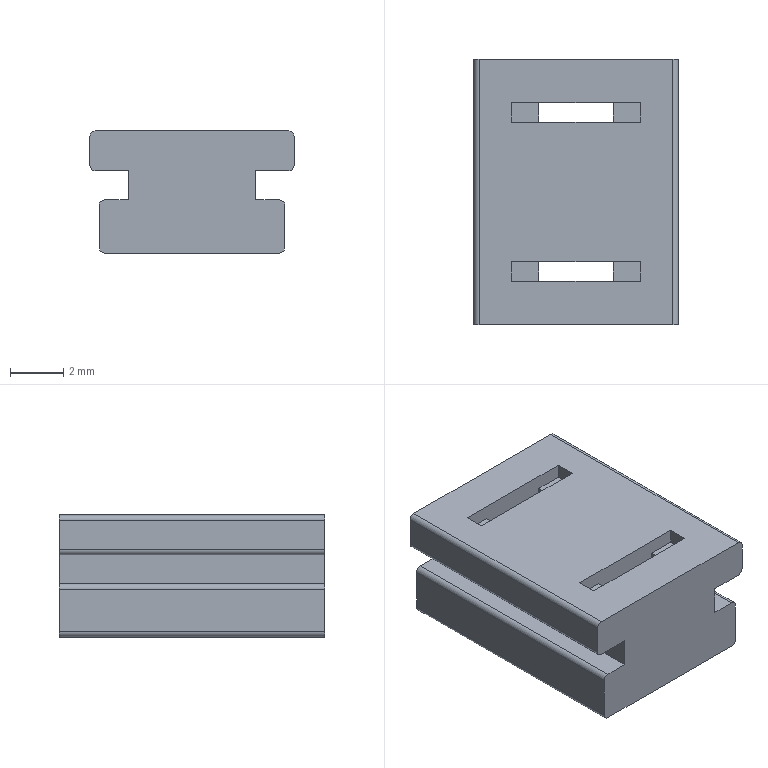Part | SolidWorks | features BaseBody 1 | 1 solid | 38 faces | box 7.7 x 10 x 4.6 mm | volume 286.602 mm3 | plane 30 | cylinder 8 | commonest cylinder face diameters 0.4 x8
STEP:
#1=CARTESIAN_POINT('',(2.425,3.375,1.5));
#2=VERTEX_POINT('',#1);
#3=CARTESIAN_POINT('',(2.425,2.625,1.5));
#4=VERTEX_POINT('',#3);
#5=CARTESIAN_POINT('',(2.425,-5.,1.5));
#6=DIRECTION('',(0.,-1.,0.));
#7=VECTOR('',#6,1000.);
#8=LINE('',#5,#7);
#9=EDGE_CURVE('',#2,#4,#8,.T.);
#10=ORIENTED_EDGE('',*,*,#9,.T.);
#11=CARTESIAN_POINT('',(-2.425,2.625,1.5));
#12=VERTEX_POINT('',#11);
#13=CARTESIAN_POINT('',(-3.85,2.625,1.5));
#14=DIRECTION('',(-1.,0.,0.));
#15=VECTOR('',#14,1000.);
#16=LINE('',#13,#15);
#17=EDGE_CURVE('',#4,#12,#16,.T.);
#18=ORIENTED_EDGE('',*,*,#17,.T.);
#19=CARTESIAN_POINT('',(-2.425,3.375,1.5));
#20=VERTEX_POINT('',#19);
#21=CARTESIAN_POINT('',(-2.425,-5.,1.5));
#22=DIRECTION('',(0.,1.,0.));
#23=VECTOR('',#22,1000.);
#24=LINE('',#21,#23);
#25=EDGE_CURVE('',#12,#20,#24,.T.);
#26=ORIENTED_EDGE('',*,*,#25,.T.);
#27=CARTESIAN_POINT('',(-3.85,3.375,1.5));
#28=DIRECTION('',(1.,0.,0.));
#29=VECTOR('',#28,1000.);
#30=LINE('',#27,#29);
#31=EDGE_CURVE('',#20,#2,#30,.T.);
#32=ORIENTED_EDGE('',*,*,#31,.T.);
#33=EDGE_LOOP('',(#10,#18,#26,#32));
#34=FACE_BOUND('',#33,.T.);
#35=CARTESIAN_POINT('',(2.425,-2.625,1.5));
#36=VERTEX_POINT('',#35);
#37=CARTESIAN_POINT('',(2.425,-3.375,1.5));
#38=VERTEX_POINT('',#37);
#39=CARTESIAN_POINT('',(2.425,-5.,1.5));
#40=DIRECTION('',(0.,-1.,0.));
#41=VECTOR('',#40,1000.);
#42=LINE('',#39,#41);
#43=EDGE_CURVE('',#36,#38,#42,.T.);
#44=ORIENTED_EDGE('',*,*,#43,.T.);
#45=CARTESIAN_POINT('',(-2.425,-3.375,1.5));
#46=VERTEX_POINT('',#45);
#47=CARTESIAN_POINT('',(-3.85,-3.375,1.5));
#48=DIRECTION('',(-1.,0.,0.));
#49=VECTOR('',#48,1000.);
#50=LINE('',#47,#49);
#51=EDGE_CURVE('',#38,#46,#50,.T.);
#52=ORIENTED_EDGE('',*,*,#51,.T.);
#53=CARTESIAN_POINT('',(-2.425,-2.625,1.5));
#54=VERTEX_POINT('',#53);
#55=CARTESIAN_POINT('',(-2.425,-5.,1.5));
#56=DIRECTION('',(0.,1.,0.));
#57=VECTOR('',#56,1000.);
#58=LINE('',#55,#57);
#59=EDGE_CURVE('',#46,#54,#58,.T.);
#60=ORIENTED_EDGE('',*,*,#59,.T.);
#61=CARTESIAN_POINT('',(-3.85,-2.625,1.5));
#62=DIRECTION('',(1.,0.,0.));
#63=VECTOR('',#62,1000.);
#64=LINE('',#61,#63);
#65=EDGE_CURVE('',#54,#36,#64,.T.);
#66=ORIENTED_EDGE('',*,*,#65,.T.);
#67=EDGE_LOOP('',(#44,#52,#60,#66));
#68=FACE_BOUND('',#67,.T.);
#69=CARTESIAN_POINT('',(-3.65,-5.,1.5));
#70=VERTEX_POINT('',#69);
#71=CARTESIAN_POINT('',(3.65,-5.,1.5));
#72=VERTEX_POINT('',#71);
#73=CARTESIAN_POINT('',(-3.85,-5.,1.5));
#74=DIRECTION('',(1.,0.,0.));
#75=VECTOR('',#74,1000.);
#76=LINE('',#73,#75);
#77=EDGE_CURVE('',#70,#72,#76,.T.);
#78=ORIENTED_EDGE('',*,*,#77,.T.);
#79=CARTESIAN_POINT('',(3.65,5.,1.5));
#80=VERTEX_POINT('',#79);
#81=CARTESIAN_POINT('',(3.65,-5.,1.5));
#82=DIRECTION('',(0.,1.,0.));
#83=VECTOR('',#82,1000.);
#84=LINE('',#81,#83);
#85=EDGE_CURVE('',#72,#80,#84,.T.);
#86=ORIENTED_EDGE('',*,*,#85,.T.);
#87=CARTESIAN_POINT('',(-3.65,5.,1.5));
#88=VERTEX_POINT('',#87);
#89=CARTESIAN_POINT('',(-3.85,5.,1.5));
#90=DIRECTION('',(-1.,0.,0.));
#91=VECTOR('',#90,1000.);
#92=LINE('',#89,#91);
#93=EDGE_CURVE('',#80,#88,#92,.T.);
#94=ORIENTED_EDGE('',*,*,#93,.T.);
#95=CARTESIAN_POINT('',(-3.65,-5.,1.5));
#96=DIRECTION('',(0.,-1.,0.));
#97=VECTOR('',#96,1000.);
#98=LINE('',#95,#97);
#99=EDGE_CURVE('',#88,#70,#98,.T.);
#100=ORIENTED_EDGE('',*,*,#99,.T.);
#101=EDGE_LOOP('',(#78,#86,#94,#100));
#102=FACE_OUTER_BOUND('',#101,.T.);
#103=CARTESIAN_POINT('',(-3.85,-5.,1.5));
#104=DIRECTION('',(0.,0.,1.));
#105=DIRECTION('',(1.,0.,0.));
#106=AXIS2_PLACEMENT_3D('',#103,#104,#105);
#107=PLANE('',#106);
#108=ADVANCED_FACE('',(#34,#68,#102),#107,.T.);
#109=CARTESIAN_POINT('',(1.4,2.625,0.95));
#110=VERTEX_POINT('',#109);
#111=CARTESIAN_POINT('',(2.425,2.625,0.95));
#112=VERTEX_POINT('',#111);
#113=CARTESIAN_POINT('',(-1.4,2.625,0.95));
#114=DIRECTION('',(1.,0.,0.));
#115=VECTOR('',#114,1000.);
#116=LINE('',#113,#115);
#117=EDGE_CURVE('',#110,#112,#116,.T.);
#118=ORIENTED_EDGE('',*,*,#117,.F.);
#119=CARTESIAN_POINT('',(1.4,2.625,-3.1));
#120=VERTEX_POINT('',#119);
#121=CARTESIAN_POINT('',(1.4,2.625,1.5));
#122=DIRECTION('',(0.,0.,1.));
#123=VECTOR('',#122,1000.);
#124=LINE('',#121,#123);
#125=EDGE_CURVE('',#120,#110,#124,.T.);
#126=ORIENTED_EDGE('',*,*,#125,.F.);
#127=CARTESIAN_POINT('',(-1.4,2.625,-3.1));
#128=VERTEX_POINT('',#127);
#129=CARTESIAN_POINT('',(-1.4,2.625,-3.1));
#130=DIRECTION('',(1.,0.,0.));
#131=VECTOR('',#130,1000.);
#132=LINE('',#129,#131);
#133=EDGE_CURVE('',#128,#120,#132,.T.);
#134=ORIENTED_EDGE('',*,*,#133,.F.);
#135=CARTESIAN_POINT('',(-1.4,2.625,0.95));
#136=VERTEX_POINT('',#135);
#137=CARTESIAN_POINT('',(-1.4,2.625,1.5));
#138=DIRECTION('',(0.,0.,-1.));
#139=VECTOR('',#138,1000.);
#140=LINE('',#137,#139);
#141=EDGE_CURVE('',#136,#128,#140,.T.);
#142=ORIENTED_EDGE('',*,*,#141,.F.);
#143=CARTESIAN_POINT('',(-2.425,2.625,0.95));
#144=VERTEX_POINT('',#143);
#145=CARTESIAN_POINT('',(-1.4,2.625,0.95));
#146=DIRECTION('',(1.,0.,0.));
#147=VECTOR('',#146,1000.);
#148=LINE('',#145,#147);
#149=EDGE_CURVE('',#144,#136,#148,.T.);
#150=ORIENTED_EDGE('',*,*,#149,.F.);
#151=CARTESIAN_POINT('',(-2.425,2.625,1.5));
#152=DIRECTION('',(0.,0.,-1.));
#153=VECTOR('',#152,1000.);
#154=LINE('',#151,#153);
#155=EDGE_CURVE('',#12,#144,#154,.T.);
#156=ORIENTED_EDGE('',*,*,#155,.F.);
#157=ORIENTED_EDGE('',*,*,#17,.F.);
#158=CARTESIAN_POINT('',(2.425,2.625,1.5));
#159=DIRECTION('',(0.,0.,1.));
#160=VECTOR('',#159,1000.);
#161=LINE('',#158,#160);
#162=EDGE_CURVE('',#112,#4,#161,.T.);
#163=ORIENTED_EDGE('',*,*,#162,.F.);
#164=EDGE_LOOP('',(#118,#126,#134,#142,#150,#156,#157,#163));
#165=FACE_OUTER_BOUND('',#164,.T.);
#166=CARTESIAN_POINT('',(-1.4,2.625,1.5));
#167=DIRECTION('',(0.,-1.,0.));
#168=DIRECTION('',(0.,0.,-1.));
#169=AXIS2_PLACEMENT_3D('',#166,#167,#168);
#170=PLANE('',#169);
#171=ADVANCED_FACE('',(#165),#170,.F.);
#172=CARTESIAN_POINT('',(2.425,3.375,0.95));
#173=VERTEX_POINT('',#172);
#174=CARTESIAN_POINT('',(2.425,2.625,0.95));
#175=DIRECTION('',(0.,1.,0.));
#176=VECTOR('',#175,1000.);
#177=LINE('',#174,#176);
#178=EDGE_CURVE('',#112,#173,#177,.T.);
#179=ORIENTED_EDGE('',*,*,#178,.F.);
#180=ORIENTED_EDGE('',*,*,#162,.T.);
#181=ORIENTED_EDGE('',*,*,#9,.F.);
#182=CARTESIAN_POINT('',(2.425,3.375,1.5));
#183=DIRECTION('',(0.,0.,1.));
#184=VECTOR('',#183,1000.);
#185=LINE('',#182,#184);
#186=EDGE_CURVE('',#173,#2,#185,.T.);
#187=ORIENTED_EDGE('',*,*,#186,.F.);
#188=EDGE_LOOP('',(#179,#180,#181,#187));
#189=FACE_OUTER_BOUND('',#188,.T.);
#190=CARTESIAN_POINT('',(2.425,2.625,1.5));
#191=DIRECTION('',(1.,0.,0.));
#192=DIRECTION('',(0.,0.,-1.));
#193=AXIS2_PLACEMENT_3D('',#190,#191,#192);
#194=PLANE('',#193);
#195=ADVANCED_FACE('',(#189),#194,.F.);
#196=CARTESIAN_POINT('',(1.4,3.375,0.95));
#197=VERTEX_POINT('',#196);
#198=CARTESIAN_POINT('',(1.4,3.375,-3.1));
#199=VERTEX_POINT('',#198);
#200=CARTESIAN_POINT('',(1.4,3.375,1.5));
#201=DIRECTION('',(0.,0.,-1.));
#202=VECTOR('',#201,1000.);
#203=LINE('',#200,#202);
#204=EDGE_CURVE('',#197,#199,#203,.T.);
#205=ORIENTED_EDGE('',*,*,#204,.F.);
#206=CARTESIAN_POINT('',(1.4,3.375,0.95));
#207=DIRECTION('',(-1.,0.,0.));
#208=VECTOR('',#207,1000.);
#209=LINE('',#206,#208);
#210=EDGE_CURVE('',#173,#197,#209,.T.);
#211=ORIENTED_EDGE('',*,*,#210,.F.);
#212=ORIENTED_EDGE('',*,*,#186,.T.);
#213=ORIENTED_EDGE('',*,*,#31,.F.);
#214=CARTESIAN_POINT('',(-2.425,3.375,0.95));
#215=VERTEX_POINT('',#214);
#216=CARTESIAN_POINT('',(-2.425,3.375,1.5));
#217=DIRECTION('',(0.,0.,1.));
#218=VECTOR('',#217,1000.);
#219=LINE('',#216,#218);
#220=EDGE_CURVE('',#215,#20,#219,.T.);
#221=ORIENTED_EDGE('',*,*,#220,.F.);
#222=CARTESIAN_POINT('',(-1.4,3.375,0.95));
#223=VERTEX_POINT('',#222);
#224=CARTESIAN_POINT('',(1.4,3.375,0.95));
#225=DIRECTION('',(-1.,0.,0.));
#226=VECTOR('',#225,1000.);
#227=LINE('',#224,#226);
#228=EDGE_CURVE('',#223,#215,#227,.T.);
#229=ORIENTED_EDGE('',*,*,#228,.F.);
#230=CARTESIAN_POINT('',(-1.4,3.375,-3.1));
#231=VERTEX_POINT('',#230);
#232=CARTESIAN_POINT('',(-1.4,3.375,1.5));
#233=DIRECTION('',(0.,0.,1.));
#234=VECTOR('',#233,1000.);
#235=LINE('',#232,#234);
#236=EDGE_CURVE('',#231,#223,#235,.T.);
#237=ORIENTED_EDGE('',*,*,#236,.F.);
#238=CARTESIAN_POINT('',(1.4,3.375,-3.1));
#239=DIRECTION('',(-1.,0.,0.));
#240=VECTOR('',#239,1000.);
#241=LINE('',#238,#240);
#242=EDGE_CURVE('',#199,#231,#241,.T.);
#243=ORIENTED_EDGE('',*,*,#242,.F.);
#244=EDGE_LOOP('',(#205,#211,#212,#213,#221,#229,#237,#243));
#245=FACE_OUTER_BOUND('',#244,.T.);
#246=CARTESIAN_POINT('',(1.4,3.375,1.5));
#247=DIRECTION('',(0.,1.,0.));
#248=DIRECTION('',(0.,0.,1.));
#249=AXIS2_PLACEMENT_3D('',#246,#247,#248);
#250=PLANE('',#249);
#251=ADVANCED_FACE('',(#245),#250,.F.);
#252=CARTESIAN_POINT('',(-2.425,3.375,0.95));
#253=DIRECTION('',(0.,-1.,0.));
#254=VECTOR('',#253,1000.);
#255=LINE('',#252,#254);
#256=EDGE_CURVE('',#215,#144,#255,.T.);
#257=ORIENTED_EDGE('',*,*,#256,.F.);
#258=ORIENTED_EDGE('',*,*,#220,.T.);
#259=ORIENTED_EDGE('',*,*,#25,.F.);
#260=ORIENTED_EDGE('',*,*,#155,.T.);
#261=EDGE_LOOP('',(#257,#258,#259,#260));
#262=FACE_OUTER_BOUND('',#261,.T.);
#263=CARTESIAN_POINT('',(-2.425,3.375,1.5));
#264=DIRECTION('',(-1.,0.,0.));
#265=DIRECTION('',(0.,0.,1.));
#266=AXIS2_PLACEMENT_3D('',#263,#264,#265);
#267=PLANE('',#266);
#268=ADVANCED_FACE('',(#262),#267,.F.);
#269=CARTESIAN_POINT('',(1.4,-3.375,0.95));
#270=VERTEX_POINT('',#269);
#271=CARTESIAN_POINT('',(2.425,-3.375,0.95));
#272=VERTEX_POINT('',#271);
#273=CARTESIAN_POINT('',(-1.4,-3.375,0.95));
#274=DIRECTION('',(1.,0.,0.));
#275=VECTOR('',#274,1000.);
#276=LINE('',#273,#275);
#277=EDGE_CURVE('',#270,#272,#276,.T.);
#278=ORIENTED_EDGE('',*,*,#277,.F.);
#279=CARTESIAN_POINT('',(1.4,-3.375,-3.1));
#280=VERTEX_POINT('',#279);
#281=CARTESIAN_POINT('',(1.4,-3.375,1.5));
#282=DIRECTION('',(0.,0.,1.));
#283=VECTOR('',#282,1000.);
#284=LINE('',#281,#283);
#285=EDGE_CURVE('',#280,#270,#284,.T.);
#286=ORIENTED_EDGE('',*,*,#285,.F.);
#287=CARTESIAN_POINT('',(-1.4,-3.375,-3.1));
#288=VERTEX_POINT('',#287);
#289=CARTESIAN_POINT('',(-1.4,-3.375,-3.1));
#290=DIRECTION('',(1.,0.,0.));
#291=VECTOR('',#290,1000.);
#292=LINE('',#289,#291);
#293=EDGE_CURVE('',#288,#280,#292,.T.);
#294=ORIENTED_EDGE('',*,*,#293,.F.);
#295=CARTESIAN_POINT('',(-1.4,-3.375,0.95));
#296=VERTEX_POINT('',#295);
#297=CARTESIAN_POINT('',(-1.4,-3.375,1.5));
#298=DIRECTION('',(0.,0.,-1.));
#299=VECTOR('',#298,1000.);
#300=LINE('',#297,#299);
#301=EDGE_CURVE('',#296,#288,#300,.T.);
#302=ORIENTED_EDGE('',*,*,#301,.F.);
#303=CARTESIAN_POINT('',(-2.425,-3.375,0.95));
#304=VERTEX_POINT('',#303);
#305=CARTESIAN_POINT('',(-1.4,-3.375,0.95));
#306=DIRECTION('',(1.,0.,0.));
#307=VECTOR('',#306,1000.);
#308=LINE('',#305,#307);
#309=EDGE_CURVE('',#304,#296,#308,.T.);
#310=ORIENTED_EDGE('',*,*,#309,.F.);
#311=CARTESIAN_POINT('',(-2.425,-3.375,1.5));
#312=DIRECTION('',(0.,0.,-1.));
#313=VECTOR('',#312,1000.);
#314=LINE('',#311,#313);
#315=EDGE_CURVE('',#46,#304,#314,.T.);
#316=ORIENTED_EDGE('',*,*,#315,.F.);
#317=ORIENTED_EDGE('',*,*,#51,.F.);
#318=CARTESIAN_POINT('',(2.425,-3.375,1.5));
#319=DIRECTION('',(0.,0.,1.));
#320=VECTOR('',#319,1000.);
#321=LINE('',#318,#320);
#322=EDGE_CURVE('',#272,#38,#321,.T.);
#323=ORIENTED_EDGE('',*,*,#322,.F.);
#324=EDGE_LOOP('',(#278,#286,#294,#302,#310,#316,#317,#323));
#325=FACE_OUTER_BOUND('',#324,.T.);
#326=CARTESIAN_POINT('',(-1.4,-3.375,1.5));
#327=DIRECTION('',(0.,-1.,0.));
#328=DIRECTION('',(0.,0.,-1.));
#329=AXIS2_PLACEMENT_3D('',#326,#327,#328);
#330=PLANE('',#329);
#331=ADVANCED_FACE('',(#325),#330,.F.);
#332=CARTESIAN_POINT('',(2.425,-2.625,0.95));
#333=VERTEX_POINT('',#332);
#334=CARTESIAN_POINT('',(2.425,-3.375,0.95));
#335=DIRECTION('',(0.,1.,0.));
#336=VECTOR('',#335,1000.);
#337=LINE('',#334,#336);
#338=EDGE_CURVE('',#272,#333,#337,.T.);
#339=ORIENTED_EDGE('',*,*,#338,.F.);
#340=ORIENTED_EDGE('',*,*,#322,.T.);
#341=ORIENTED_EDGE('',*,*,#43,.F.);
#342=CARTESIAN_POINT('',(2.425,-2.625,1.5));
#343=DIRECTION('',(0.,0.,1.));
#344=VECTOR('',#343,1000.);
#345=LINE('',#342,#344);
#346=EDGE_CURVE('',#333,#36,#345,.T.);
#347=ORIENTED_EDGE('',*,*,#346,.F.);
#348=EDGE_LOOP('',(#339,#340,#341,#347));
#349=FACE_OUTER_BOUND('',#348,.T.);
#350=CARTESIAN_POINT('',(2.425,-3.375,1.5));
#351=DIRECTION('',(1.,0.,0.));
#352=DIRECTION('',(0.,0.,-1.));
#353=AXIS2_PLACEMENT_3D('',#350,#351,#352);
#354=PLANE('',#353);
#355=ADVANCED_FACE('',(#349),#354,.F.);
#356=CARTESIAN_POINT('',(1.4,-2.625,0.95));
#357=VERTEX_POINT('',#356);
#358=CARTESIAN_POINT('',(1.4,-2.625,-3.1));
#359=VERTEX_POINT('',#358);
#360=CARTESIAN_POINT('',(1.4,-2.625,1.5));
#361=DIRECTION('',(0.,0.,-1.));
#362=VECTOR('',#361,1000.);
#363=LINE('',#360,#362);
#364=EDGE_CURVE('',#357,#359,#363,.T.);
#365=ORIENTED_EDGE('',*,*,#364,.F.);
#366=CARTESIAN_POINT('',(1.4,-2.625,0.95));
#367=DIRECTION('',(-1.,0.,0.));
#368=VECTOR('',#367,1000.);
#369=LINE('',#366,#368);
#370=EDGE_CURVE('',#333,#357,#369,.T.);
#371=ORIENTED_EDGE('',*,*,#370,.F.);
#372=ORIENTED_EDGE('',*,*,#346,.T.);
#373=ORIENTED_EDGE('',*,*,#65,.F.);
#374=CARTESIAN_POINT('',(-2.425,-2.625,0.95));
#375=VERTEX_POINT('',#374);
#376=CARTESIAN_POINT('',(-2.425,-2.625,1.5));
#377=DIRECTION('',(0.,0.,1.));
#378=VECTOR('',#377,1000.);
#379=LINE('',#376,#378);
#380=EDGE_CURVE('',#375,#54,#379,.T.);
#381=ORIENTED_EDGE('',*,*,#380,.F.);
#382=CARTESIAN_POINT('',(-1.4,-2.625,0.95));
#383=VERTEX_POINT('',#382);
#384=CARTESIAN_POINT('',(1.4,-2.625,0.95));
#385=DIRECTION('',(-1.,0.,0.));
#386=VECTOR('',#385,1000.);
#387=LINE('',#384,#386);
#388=EDGE_CURVE('',#383,#375,#387,.T.);
#389=ORIENTED_EDGE('',*,*,#388,.F.);
#390=CARTESIAN_POINT('',(-1.4,-2.625,-3.1));
#391=VERTEX_POINT('',#390);
#392=CARTESIAN_POINT('',(-1.4,-2.625,1.5));
#393=DIRECTION('',(0.,0.,1.));
#394=VECTOR('',#393,1000.);
#395=LINE('',#392,#394);
#396=EDGE_CURVE('',#391,#383,#395,.T.);
#397=ORIENTED_EDGE('',*,*,#396,.F.);
#398=CARTESIAN_POINT('',(1.4,-2.625,-3.1));
#399=DIRECTION('',(-1.,0.,0.));
#400=VECTOR('',#399,1000.);
#401=LINE('',#398,#400);
#402=EDGE_CURVE('',#359,#391,#401,.T.);
#403=ORIENTED_EDGE('',*,*,#402,.F.);
#404=EDGE_LOOP('',(#365,#371,#372,#373,#381,#389,#397,#403));
#405=FACE_OUTER_BOUND('',#404,.T.);
#406=CARTESIAN_POINT('',(1.4,-2.625,1.5));
#407=DIRECTION('',(0.,1.,0.));
#408=DIRECTION('',(0.,0.,1.));
#409=AXIS2_PLACEMENT_3D('',#406,#407,#408);
#410=PLANE('',#409);
#411=ADVANCED_FACE('',(#405),#410,.F.);
#412=CARTESIAN_POINT('',(-2.425,-2.625,0.95));
#413=DIRECTION('',(0.,-1.,0.));
#414=VECTOR('',#413,1000.);
#415=LINE('',#412,#414);
#416=EDGE_CURVE('',#375,#304,#415,.T.);
#417=ORIENTED_EDGE('',*,*,#416,.F.);
#418=ORIENTED_EDGE('',*,*,#380,.T.);
#419=ORIENTED_EDGE('',*,*,#59,.F.);
#420=ORIENTED_EDGE('',*,*,#315,.T.);
#421=EDGE_LOOP('',(#417,#418,#419,#420));
#422=FACE_OUTER_BOUND('',#421,.T.);
#423=CARTESIAN_POINT('',(-2.425,-2.625,1.5));
#424=DIRECTION('',(-1.,0.,0.));
#425=DIRECTION('',(0.,0.,1.));
#426=AXIS2_PLACEMENT_3D('',#423,#424,#425);
#427=PLANE('',#426);
#428=ADVANCED_FACE('',(#422),#427,.F.);
#429=ORIENTED_EDGE('',*,*,#85,.F.);
#430=CARTESIAN_POINT('',(3.85,-5.,1.3));
#431=VERTEX_POINT('',#430);
#432=CARTESIAN_POINT('',(3.65,-5.,1.3));
#433=DIRECTION('',(0.,1.,0.));
#434=DIRECTION('',(0.,0.,-1.));
#435=AXIS2_PLACEMENT_3D('',#432,#433,#434);
#436=CIRCLE('',#435,0.2);
#437=EDGE_CURVE('',#72,#431,#436,.T.);
#438=ORIENTED_EDGE('',*,*,#437,.T.);
#439=CARTESIAN_POINT('',(3.85,5.,1.3));
#440=VERTEX_POINT('',#439);
#441=CARTESIAN_POINT('',(3.85,18.036,1.3));
#442=DIRECTION('',(0.,1.,0.));
#443=VECTOR('',#442,1000.);
#444=LINE('',#441,#443);
#445=EDGE_CURVE('',#431,#440,#444,.T.);
#446=ORIENTED_EDGE('',*,*,#445,.T.);
#447=CARTESIAN_POINT('',(3.65,5.,1.3));
#448=DIRECTION('',(0.,-1.,0.));
#449=DIRECTION('',(0.,0.,-1.));
#450=AXIS2_PLACEMENT_3D('',#447,#448,#449);
#451=CIRCLE('',#450,0.2);
#452=EDGE_CURVE('',#440,#80,#451,.T.);
#453=ORIENTED_EDGE('',*,*,#452,.T.);
#454=EDGE_LOOP('',(#429,#438,#446,#453));
#455=FACE_OUTER_BOUND('',#454,.T.);
#456=CARTESIAN_POINT('',(3.65,18.036,1.3));
#457=DIRECTION('',(0.,-1.,0.));
#458=DIRECTION('',(0.,0.,-1.));
#459=AXIS2_PLACEMENT_3D('',#456,#457,#458);
#460=CYLINDRICAL_SURFACE('',#459,0.2);
#461=ADVANCED_FACE('',(#455),#460,.T.);
#462=CARTESIAN_POINT('',(3.5,-5.,-2.9));
#463=VERTEX_POINT('',#462);
#464=CARTESIAN_POINT('',(3.3,-5.,-3.1));
#465=VERTEX_POINT('',#464);
#466=CARTESIAN_POINT('',(3.3,-5.,-2.9));
#467=DIRECTION('',(0.,1.,0.));
#468=DIRECTION('',(0.,0.,-1.));
#469=AXIS2_PLACEMENT_3D('',#466,#467,#468);
#470=CIRCLE('',#469,0.2);
#471=EDGE_CURVE('',#463,#465,#470,.T.);
#472=ORIENTED_EDGE('',*,*,#471,.F.);
#473=CARTESIAN_POINT('',(3.5,-5.,-1.3));
#474=VERTEX_POINT('',#473);
#475=CARTESIAN_POINT('',(3.5,-5.,-1.1));
#476=DIRECTION('',(0.,0.,-1.));
#477=VECTOR('',#476,1000.);
#478=LINE('',#475,#477);
#479=EDGE_CURVE('',#474,#463,#478,.T.);
#480=ORIENTED_EDGE('',*,*,#479,.F.);
#481=CARTESIAN_POINT('',(3.3,-5.,-1.1));
#482=VERTEX_POINT('',#481);
#483=CARTESIAN_POINT('',(3.3,-5.,-1.3));
#484=DIRECTION('',(0.,1.,0.));
#485=DIRECTION('',(0.,0.,-1.));
#486=AXIS2_PLACEMENT_3D('',#483,#484,#485);
#487=CIRCLE('',#486,0.2);
#488=EDGE_CURVE('',#482,#474,#487,.T.);
#489=ORIENTED_EDGE('',*,*,#488,.F.);
#490=CARTESIAN_POINT('',(2.4,-5.,-1.1));
#491=VERTEX_POINT('',#490);
#492=CARTESIAN_POINT('',(-3.5,-5.,-1.1));
#493=DIRECTION('',(1.,0.,0.));
#494=VECTOR('',#493,1000.);
#495=LINE('',#492,#494);
#496=EDGE_CURVE('',#491,#482,#495,.T.);
#497=ORIENTED_EDGE('',*,*,#496,.F.);
#498=CARTESIAN_POINT('',(2.4,-5.,0.));
#499=VERTEX_POINT('',#498);
#500=CARTESIAN_POINT('',(2.4,-5.,0.));
#501=DIRECTION('',(0.,0.,-1.));
#502=VECTOR('',#501,1000.);
#503=LINE('',#500,#502);
#504=EDGE_CURVE('',#499,#491,#503,.T.);
#505=ORIENTED_EDGE('',*,*,#504,.F.);
#506=CARTESIAN_POINT('',(3.65,-5.,0.));
#507=VERTEX_POINT('',#506);
#508=CARTESIAN_POINT('',(3.85,-5.,0.));
#509=DIRECTION('',(-1.,0.,0.));
#510=VECTOR('',#509,1000.);
#511=LINE('',#508,#510);
#512=EDGE_CURVE('',#507,#499,#511,.T.);
#513=ORIENTED_EDGE('',*,*,#512,.F.);
#514=CARTESIAN_POINT('',(3.85,-5.,0.2));
#515=VERTEX_POINT('',#514);
#516=CARTESIAN_POINT('',(3.65,-5.,0.2));
#517=DIRECTION('',(0.,1.,0.));
#518=DIRECTION('',(0.,0.,-1.));
#519=AXIS2_PLACEMENT_3D('',#516,#517,#518);
#520=CIRCLE('',#519,0.2);
#521=EDGE_CURVE('',#515,#507,#520,.T.);
#522=ORIENTED_EDGE('',*,*,#521,.F.);
#523=CARTESIAN_POINT('',(3.85,-5.,0.));
#524=DIRECTION('',(0.,0.,-1.));
#525=VECTOR('',#524,1000.);
#526=LINE('',#523,#525);
#527=EDGE_CURVE('',#431,#515,#526,.T.);
#528=ORIENTED_EDGE('',*,*,#527,.F.);
#529=ORIENTED_EDGE('',*,*,#437,.F.);
#530=ORIENTED_EDGE('',*,*,#77,.F.);
#531=CARTESIAN_POINT('',(-3.85,-5.,1.3));
#532=VERTEX_POINT('',#531);
#533=CARTESIAN_POINT('',(-3.65,-5.,1.3));
#534=DIRECTION('',(0.,1.,0.));
#535=DIRECTION('',(0.,0.,-1.));
#536=AXIS2_PLACEMENT_3D('',#533,#534,#535);
#537=CIRCLE('',#536,0.2);
#538=EDGE_CURVE('',#532,#70,#537,.T.);
#539=ORIENTED_EDGE('',*,*,#538,.F.);
#540=CARTESIAN_POINT('',(-3.85,-5.,0.2));
#541=VERTEX_POINT('',#540);
#542=CARTESIAN_POINT('',(-3.85,-5.,0.));
#543=DIRECTION('',(0.,0.,1.));
#544=VECTOR('',#543,1000.);
#545=LINE('',#542,#544);
#546=EDGE_CURVE('',#541,#532,#545,.T.);
#547=ORIENTED_EDGE('',*,*,#546,.F.);
#548=CARTESIAN_POINT('',(-3.65,-5.,0.));
#549=VERTEX_POINT('',#548);
#550=CARTESIAN_POINT('',(-3.65,-5.,0.2));
#551=DIRECTION('',(0.,1.,0.));
#552=DIRECTION('',(0.,0.,-1.));
#553=AXIS2_PLACEMENT_3D('',#550,#551,#552);
#554=CIRCLE('',#553,0.2);
#555=EDGE_CURVE('',#549,#541,#554,.T.);
#556=ORIENTED_EDGE('',*,*,#555,.F.);
#557=CARTESIAN_POINT('',(-2.4,-5.,0.));
#558=VERTEX_POINT('',#557);
#559=CARTESIAN_POINT('',(3.85,-5.,0.));
#560=DIRECTION('',(-1.,0.,0.));
#561=VECTOR('',#560,1000.);
#562=LINE('',#559,#561);
#563=EDGE_CURVE('',#558,#549,#562,.T.);
#564=ORIENTED_EDGE('',*,*,#563,.F.);
#565=CARTESIAN_POINT('',(-2.4,-5.,-1.1));
#566=VERTEX_POINT('',#565);
#567=CARTESIAN_POINT('',(-2.4,-5.,-1.1));
#568=DIRECTION('',(0.,0.,1.));
#569=VECTOR('',#568,1000.);
#570=LINE('',#567,#569);
#571=EDGE_CURVE('',#566,#558,#570,.T.);
#572=ORIENTED_EDGE('',*,*,#571,.F.);
#573=CARTESIAN_POINT('',(-3.3,-5.,-1.1));
#574=VERTEX_POINT('',#573);
#575=CARTESIAN_POINT('',(-3.5,-5.,-1.1));
#576=DIRECTION('',(1.,0.,0.));
#577=VECTOR('',#576,1000.);
#578=LINE('',#575,#577);
#579=EDGE_CURVE('',#574,#566,#578,.T.);
#580=ORIENTED_EDGE('',*,*,#579,.F.);
#581=CARTESIAN_POINT('',(-3.5,-5.,-1.3));
#582=VERTEX_POINT('',#581);
#583=CARTESIAN_POINT('',(-3.3,-5.,-1.3));
#584=DIRECTION('',(0.,1.,0.));
#585=DIRECTION('',(0.,0.,-1.));
#586=AXIS2_PLACEMENT_3D('',#583,#584,#585);
#587=CIRCLE('',#586,0.2);
#588=EDGE_CURVE('',#582,#574,#587,.T.);
#589=ORIENTED_EDGE('',*,*,#588,.F.);
#590=CARTESIAN_POINT('',(-3.5,-5.,-2.9));
#591=VERTEX_POINT('',#590);
#592=CARTESIAN_POINT('',(-3.5,-5.,-3.1));
#593=DIRECTION('',(0.,0.,1.));
#594=VECTOR('',#593,1000.);
#595=LINE('',#592,#594);
#596=EDGE_CURVE('',#591,#582,#595,.T.);
#597=ORIENTED_EDGE('',*,*,#596,.F.);
#598=CARTESIAN_POINT('',(-3.3,-5.,-3.1));
#599=VERTEX_POINT('',#598);
#600=CARTESIAN_POINT('',(-3.3,-5.,-2.9));
#601=DIRECTION('',(0.,1.,0.));
#602=DIRECTION('',(0.,0.,-1.));
#603=AXIS2_PLACEMENT_3D('',#600,#601,#602);
#604=CIRCLE('',#603,0.2);
#605=EDGE_CURVE('',#599,#591,#604,.T.);
#606=ORIENTED_EDGE('',*,*,#605,.F.);
#607=CARTESIAN_POINT('',(0.,-5.,-3.1));
#608=DIRECTION('',(-1.,0.,0.));
#609=VECTOR('',#608,1000.);
#610=LINE('',#607,#609);
#611=EDGE_CURVE('',#465,#599,#610,.T.);
#612=ORIENTED_EDGE('',*,*,#611,.F.);
#613=EDGE_LOOP('',(#472,#480,#489,#497,#505,#513,#522,#528,#529,#530,#539,#547,#556,#564,#572,#580,#589,#597,#606,#612));
#614=FACE_OUTER_BOUND('',#613,.T.);
#615=CARTESIAN_POINT('',(0.,-5.,0.));
#616=DIRECTION('',(0.,1.,0.));
#617=DIRECTION('',(0.,0.,1.));
#618=AXIS2_PLACEMENT_3D('',#615,#616,#617);
#619=PLANE('',#618);
#620=ADVANCED_FACE('',(#614),#619,.F.);
#621=CARTESIAN_POINT('',(-3.85,5.,1.3));
#622=VERTEX_POINT('',#621);
#623=CARTESIAN_POINT('',(-3.85,18.036,1.3));
#624=DIRECTION('',(0.,-1.,0.));
#625=VECTOR('',#624,1000.);
#626=LINE('',#623,#625);
#627=EDGE_CURVE('',#622,#532,#626,.T.);
#628=ORIENTED_EDGE('',*,*,#627,.T.);
#629=ORIENTED_EDGE('',*,*,#538,.T.);
#630=ORIENTED_EDGE('',*,*,#99,.F.);
#631=CARTESIAN_POINT('',(-3.65,5.,1.3));
#632=DIRECTION('',(0.,-1.,0.));
#633=DIRECTION('',(0.,0.,-1.));
#634=AXIS2_PLACEMENT_3D('',#631,#632,#633);
#635=CIRCLE('',#634,0.2);
#636=EDGE_CURVE('',#88,#622,#635,.T.);
#637=ORIENTED_EDGE('',*,*,#636,.T.);
#638=EDGE_LOOP('',(#628,#629,#630,#637));
#639=FACE_OUTER_BOUND('',#638,.T.);
#640=CARTESIAN_POINT('',(-3.65,18.036,1.3));
#641=DIRECTION('',(0.,-1.,0.));
#642=DIRECTION('',(0.,0.,-1.));
#643=AXIS2_PLACEMENT_3D('',#640,#641,#642);
#644=CYLINDRICAL_SURFACE('',#643,0.2);
#645=ADVANCED_FACE('',(#639),#644,.T.);
#646=CARTESIAN_POINT('',(3.3,5.,-3.1));
#647=VERTEX_POINT('',#646);
#648=CARTESIAN_POINT('',(-3.3,5.,-3.1));
#649=VERTEX_POINT('',#648);
#650=CARTESIAN_POINT('',(0.,5.,-3.1));
#651=DIRECTION('',(-1.,0.,0.));
#652=VECTOR('',#651,1000.);
#653=LINE('',#650,#652);
#654=EDGE_CURVE('',#647,#649,#653,.T.);
#655=ORIENTED_EDGE('',*,*,#654,.T.);
#656=CARTESIAN_POINT('',(-3.5,5.,-2.9));
#657=VERTEX_POINT('',#656);
#658=CARTESIAN_POINT('',(-3.3,5.,-2.9));
#659=DIRECTION('',(0.,-1.,0.));
#660=DIRECTION('',(0.,0.,-1.));
#661=AXIS2_PLACEMENT_3D('',#658,#659,#660);
#662=CIRCLE('',#661,0.2);
#663=EDGE_CURVE('',#657,#649,#662,.T.);
#664=ORIENTED_EDGE('',*,*,#663,.F.);
#665=CARTESIAN_POINT('',(-3.5,5.,-1.3));
#666=VERTEX_POINT('',#665);
#667=CARTESIAN_POINT('',(-3.5,5.,-3.1));
#668=DIRECTION('',(0.,0.,-1.));
#669=VECTOR('',#668,1000.);
#670=LINE('',#667,#669);
#671=EDGE_CURVE('',#666,#657,#670,.T.);
#672=ORIENTED_EDGE('',*,*,#671,.F.);
#673=CARTESIAN_POINT('',(-3.3,5.,-1.1));
#674=VERTEX_POINT('',#673);
#675=CARTESIAN_POINT('',(-3.3,5.,-1.3));
#676=DIRECTION('',(0.,-1.,0.));
#677=DIRECTION('',(0.,0.,-1.));
#678=AXIS2_PLACEMENT_3D('',#675,#676,#677);
#679=CIRCLE('',#678,0.2);
#680=EDGE_CURVE('',#674,#666,#679,.T.);
#681=ORIENTED_EDGE('',*,*,#680,.F.);
#682=CARTESIAN_POINT('',(-2.4,5.,-1.1));
#683=VERTEX_POINT('',#682);
#684=CARTESIAN_POINT('',(-3.5,5.,-1.1));
#685=DIRECTION('',(-1.,0.,0.));
#686=VECTOR('',#685,1000.);
#687=LINE('',#684,#686);
#688=EDGE_CURVE('',#683,#674,#687,.T.);
#689=ORIENTED_EDGE('',*,*,#688,.F.);
#690=CARTESIAN_POINT('',(-2.4,5.,0.));
#691=VERTEX_POINT('',#690);
#692=CARTESIAN_POINT('',(-2.4,5.,-1.1));
#693=DIRECTION('',(0.,0.,-1.));
#694=VECTOR('',#693,1000.);
#695=LINE('',#692,#694);
#696=EDGE_CURVE('',#691,#683,#695,.T.);
#697=ORIENTED_EDGE('',*,*,#696,.F.);
#698=CARTESIAN_POINT('',(-3.65,5.,0.));
#699=VERTEX_POINT('',#698);
#700=CARTESIAN_POINT('',(3.85,5.,0.));
#701=DIRECTION('',(1.,0.,0.));
#702=VECTOR('',#701,1000.);
#703=LINE('',#700,#702);
#704=EDGE_CURVE('',#699,#691,#703,.T.);
#705=ORIENTED_EDGE('',*,*,#704,.F.);
#706=CARTESIAN_POINT('',(-3.85,5.,0.2));
#707=VERTEX_POINT('',#706);
#708=CARTESIAN_POINT('',(-3.65,5.,0.2));
#709=DIRECTION('',(0.,-1.,0.));
#710=DIRECTION('',(0.,0.,-1.));
#711=AXIS2_PLACEMENT_3D('',#708,#709,#710);
#712=CIRCLE('',#711,0.2);
#713=EDGE_CURVE('',#707,#699,#712,.T.);
#714=ORIENTED_EDGE('',*,*,#713,.F.);
#715=CARTESIAN_POINT('',(-3.85,5.,0.));
#716=DIRECTION('',(0.,0.,1.));
#717=VECTOR('',#716,1000.);
#718=LINE('',#715,#717);
#719=EDGE_CURVE('',#707,#622,#718,.T.);
#720=ORIENTED_EDGE('',*,*,#719,.T.);
#721=ORIENTED_EDGE('',*,*,#636,.F.);
#722=ORIENTED_EDGE('',*,*,#93,.F.);
#723=ORIENTED_EDGE('',*,*,#452,.F.);
#724=CARTESIAN_POINT('',(3.85,5.,0.2));
#725=VERTEX_POINT('',#724);
#726=CARTESIAN_POINT('',(3.85,5.,0.));
#727=DIRECTION('',(0.,0.,-1.));
#728=VECTOR('',#727,1000.);
#729=LINE('',#726,#728);
#730=EDGE_CURVE('',#440,#725,#729,.T.);
#731=ORIENTED_EDGE('',*,*,#730,.T.);
#732=CARTESIAN_POINT('',(3.65,5.,0.));
#733=VERTEX_POINT('',#732);
#734=CARTESIAN_POINT('',(3.65,5.,0.2));
#735=DIRECTION('',(0.,-1.,0.));
#736=DIRECTION('',(0.,0.,-1.));
#737=AXIS2_PLACEMENT_3D('',#734,#735,#736);
#738=CIRCLE('',#737,0.2);
#739=EDGE_CURVE('',#733,#725,#738,.T.);
#740=ORIENTED_EDGE('',*,*,#739,.F.);
#741=CARTESIAN_POINT('',(2.4,5.,0.));
#742=VERTEX_POINT('',#741);
#743=CARTESIAN_POINT('',(3.85,5.,0.));
#744=DIRECTION('',(1.,0.,0.));
#745=VECTOR('',#744,1000.);
#746=LINE('',#743,#745);
#747=EDGE_CURVE('',#742,#733,#746,.T.);
#748=ORIENTED_EDGE('',*,*,#747,.F.);
#749=CARTESIAN_POINT('',(2.4,5.,-1.1));
#750=VERTEX_POINT('',#749);
#751=CARTESIAN_POINT('',(2.4,5.,0.));
#752=DIRECTION('',(0.,0.,1.));
#753=VECTOR('',#752,1000.);
#754=LINE('',#751,#753);
#755=EDGE_CURVE('',#750,#742,#754,.T.);
#756=ORIENTED_EDGE('',*,*,#755,.F.);
#757=CARTESIAN_POINT('',(3.3,5.,-1.1));
#758=VERTEX_POINT('',#757);
#759=CARTESIAN_POINT('',(-3.5,5.,-1.1));
#760=DIRECTION('',(-1.,0.,0.));
#761=VECTOR('',#760,1000.);
#762=LINE('',#759,#761);
#763=EDGE_CURVE('',#758,#750,#762,.T.);
#764=ORIENTED_EDGE('',*,*,#763,.F.);
#765=CARTESIAN_POINT('',(3.5,5.,-1.3));
#766=VERTEX_POINT('',#765);
#767=CARTESIAN_POINT('',(3.3,5.,-1.3));
#768=DIRECTION('',(0.,-1.,0.));
#769=DIRECTION('',(0.,0.,-1.));
#770=AXIS2_PLACEMENT_3D('',#767,#768,#769);
#771=CIRCLE('',#770,0.2);
#772=EDGE_CURVE('',#766,#758,#771,.T.);
#773=ORIENTED_EDGE('',*,*,#772,.F.);
#774=CARTESIAN_POINT('',(3.5,5.,-2.9));
#775=VERTEX_POINT('',#774);
#776=CARTESIAN_POINT('',(3.5,5.,-1.1));
#777=DIRECTION('',(0.,0.,1.));
#778=VECTOR('',#777,1000.);
#779=LINE('',#776,#778);
#780=EDGE_CURVE('',#775,#766,#779,.T.);
#781=ORIENTED_EDGE('',*,*,#780,.F.);
#782=CARTESIAN_POINT('',(3.3,5.,-2.9));
#783=DIRECTION('',(0.,-1.,0.));
#784=DIRECTION('',(0.,0.,-1.));
#785=AXIS2_PLACEMENT_3D('',#782,#783,#784);
#786=CIRCLE('',#785,0.2);
#787=EDGE_CURVE('',#647,#775,#786,.T.);
#788=ORIENTED_EDGE('',*,*,#787,.F.);
#789=EDGE_LOOP('',(#655,#664,#672,#681,#689,#697,#705,#714,#720,#721,#722,#723,#731,#740,#748,#756,#764,#773,#781,#788));
#790=FACE_OUTER_BOUND('',#789,.T.);
#791=CARTESIAN_POINT('',(0.,5.,0.));
#792=DIRECTION('',(0.,1.,0.));
#793=DIRECTION('',(0.,0.,1.));
#794=AXIS2_PLACEMENT_3D('',#791,#792,#793);
#795=PLANE('',#794);
#796=ADVANCED_FACE('',(#790),#795,.T.);
#797=ORIENTED_EDGE('',*,*,#210,.T.);
#798=CARTESIAN_POINT('',(1.4,-5.,0.95));
#799=DIRECTION('',(0.,-1.,0.));
#800=VECTOR('',#799,1000.);
#801=LINE('',#798,#800);
#802=EDGE_CURVE('',#197,#110,#801,.T.);
#803=ORIENTED_EDGE('',*,*,#802,.T.);
#804=ORIENTED_EDGE('',*,*,#117,.T.);
#805=ORIENTED_EDGE('',*,*,#178,.T.);
#806=EDGE_LOOP('',(#797,#803,#804,#805));
#807=FACE_OUTER_BOUND('',#806,.T.);
#808=CARTESIAN_POINT('',(0.,-5.,0.95));
#809=DIRECTION('',(0.,0.,1.));
#810=DIRECTION('',(1.,0.,0.));
#811=AXIS2_PLACEMENT_3D('',#808,#809,#810);
#812=PLANE('',#811);
#813=ADVANCED_FACE('',(#807),#812,.T.);
#814=CARTESIAN_POINT('',(1.4,2.625,-3.1));
#815=DIRECTION('',(0.,1.,0.));
#816=VECTOR('',#815,1000.);
#817=LINE('',#814,#816);
#818=EDGE_CURVE('',#120,#199,#817,.T.);
#819=ORIENTED_EDGE('',*,*,#818,.F.);
#820=ORIENTED_EDGE('',*,*,#125,.T.);
#821=ORIENTED_EDGE('',*,*,#802,.F.);
#822=ORIENTED_EDGE('',*,*,#204,.T.);
#823=EDGE_LOOP('',(#819,#820,#821,#822));
#824=FACE_OUTER_BOUND('',#823,.T.);
#825=CARTESIAN_POINT('',(1.4,2.625,1.5));
#826=DIRECTION('',(1.,0.,0.));
#827=DIRECTION('',(0.,0.,-1.));
#828=AXIS2_PLACEMENT_3D('',#825,#826,#827);
#829=PLANE('',#828);
#830=ADVANCED_FACE('',(#824),#829,.F.);
#831=ORIENTED_EDGE('',*,*,#293,.T.);
#832=CARTESIAN_POINT('',(1.4,5.,-3.1));
#833=DIRECTION('',(0.,1.,0.));
#834=VECTOR('',#833,1000.);
#835=LINE('',#832,#834);
#836=EDGE_CURVE('',#280,#359,#835,.T.);
#837=ORIENTED_EDGE('',*,*,#836,.T.);
#838=ORIENTED_EDGE('',*,*,#402,.T.);
#839=CARTESIAN_POINT('',(-1.4,5.,-3.1));
#840=DIRECTION('',(0.,-1.,0.));
#841=VECTOR('',#840,1000.);
#842=LINE('',#839,#841);
#843=EDGE_CURVE('',#391,#288,#842,.T.);
#844=ORIENTED_EDGE('',*,*,#843,.T.);
#845=EDGE_LOOP('',(#831,#837,#838,#844));
#846=FACE_BOUND('',#845,.T.);
#847=ORIENTED_EDGE('',*,*,#818,.T.);
#848=ORIENTED_EDGE('',*,*,#242,.T.);
#849=CARTESIAN_POINT('',(-1.4,5.,-3.1));
#850=DIRECTION('',(0.,-1.,0.));
#851=VECTOR('',#850,1000.);
#852=LINE('',#849,#851);
#853=EDGE_CURVE('',#231,#128,#852,.T.);
#854=ORIENTED_EDGE('',*,*,#853,.T.);
#855=ORIENTED_EDGE('',*,*,#133,.T.);
#856=EDGE_LOOP('',(#847,#848,#854,#855));
#857=FACE_BOUND('',#856,.T.);
#858=ORIENTED_EDGE('',*,*,#611,.T.);
#859=CARTESIAN_POINT('',(-3.3,5.,-3.1));
#860=DIRECTION('',(0.,1.,0.));
#861=VECTOR('',#860,1000.);
#862=LINE('',#859,#861);
#863=EDGE_CURVE('',#599,#649,#862,.T.);
#864=ORIENTED_EDGE('',*,*,#863,.T.);
#865=ORIENTED_EDGE('',*,*,#654,.F.);
#866=CARTESIAN_POINT('',(3.3,5.,-3.1));
#867=DIRECTION('',(0.,-1.,0.));
#868=VECTOR('',#867,1000.);
#869=LINE('',#866,#868);
#870=EDGE_CURVE('',#647,#465,#869,.T.);
#871=ORIENTED_EDGE('',*,*,#870,.T.);
#872=EDGE_LOOP('',(#858,#864,#865,#871));
#873=FACE_OUTER_BOUND('',#872,.T.);
#874=CARTESIAN_POINT('',(3.5,5.,-3.1));
#875=DIRECTION('',(0.,0.,-1.));
#876=DIRECTION('',(-1.,0.,0.));
#877=AXIS2_PLACEMENT_3D('',#874,#875,#876);
#878=PLANE('',#877);
#879=ADVANCED_FACE('',(#846,#857,#873),#878,.T.);
#880=ORIENTED_EDGE('',*,*,#853,.F.);
#881=ORIENTED_EDGE('',*,*,#236,.T.);
#882=CARTESIAN_POINT('',(-1.4,3.375,0.95));
#883=DIRECTION('',(0.,1.,0.));
#884=VECTOR('',#883,1000.);
#885=LINE('',#882,#884);
#886=EDGE_CURVE('',#136,#223,#885,.T.);
#887=ORIENTED_EDGE('',*,*,#886,.F.);
#888=ORIENTED_EDGE('',*,*,#141,.T.);
#889=EDGE_LOOP('',(#880,#881,#887,#888));
#890=FACE_OUTER_BOUND('',#889,.T.);
#891=CARTESIAN_POINT('',(-1.4,3.375,1.5));
#892=DIRECTION('',(-1.,0.,0.));
#893=DIRECTION('',(0.,0.,1.));
#894=AXIS2_PLACEMENT_3D('',#891,#892,#893);
#895=PLANE('',#894);
#896=ADVANCED_FACE('',(#890),#895,.F.);
#897=ORIENTED_EDGE('',*,*,#149,.T.);
#898=ORIENTED_EDGE('',*,*,#886,.T.);
#899=ORIENTED_EDGE('',*,*,#228,.T.);
#900=ORIENTED_EDGE('',*,*,#256,.T.);
#901=EDGE_LOOP('',(#897,#898,#899,#900));
#902=FACE_OUTER_BOUND('',#901,.T.);
#903=CARTESIAN_POINT('',(0.,-5.,0.95));
#904=DIRECTION('',(0.,0.,1.));
#905=DIRECTION('',(1.,0.,0.));
#906=AXIS2_PLACEMENT_3D('',#903,#904,#905);
#907=PLANE('',#906);
#908=ADVANCED_FACE('',(#902),#907,.T.);
#909=ORIENTED_EDGE('',*,*,#370,.T.);
#910=CARTESIAN_POINT('',(1.4,-5.,0.95));
#911=DIRECTION('',(0.,-1.,0.));
#912=VECTOR('',#911,1000.);
#913=LINE('',#910,#912);
#914=EDGE_CURVE('',#357,#270,#913,.T.);
#915=ORIENTED_EDGE('',*,*,#914,.T.);
#916=ORIENTED_EDGE('',*,*,#277,.T.);
#917=ORIENTED_EDGE('',*,*,#338,.T.);
#918=EDGE_LOOP('',(#909,#915,#916,#917));
#919=FACE_OUTER_BOUND('',#918,.T.);
#920=CARTESIAN_POINT('',(0.,-5.,0.95));
#921=DIRECTION('',(0.,0.,1.));
#922=DIRECTION('',(1.,0.,0.));
#923=AXIS2_PLACEMENT_3D('',#920,#921,#922);
#924=PLANE('',#923);
#925=ADVANCED_FACE('',(#919),#924,.T.);
#926=ORIENTED_EDGE('',*,*,#836,.F.);
#927=ORIENTED_EDGE('',*,*,#285,.T.);
#928=ORIENTED_EDGE('',*,*,#914,.F.);
#929=ORIENTED_EDGE('',*,*,#364,.T.);
#930=EDGE_LOOP('',(#926,#927,#928,#929));
#931=FACE_OUTER_BOUND('',#930,.T.);
#932=CARTESIAN_POINT('',(1.4,-3.375,1.5));
#933=DIRECTION('',(1.,0.,0.));
#934=DIRECTION('',(0.,0.,-1.));
#935=AXIS2_PLACEMENT_3D('',#932,#933,#934);
#936=PLANE('',#935);
#937=ADVANCED_FACE('',(#931),#936,.F.);
#938=ORIENTED_EDGE('',*,*,#843,.F.);
#939=ORIENTED_EDGE('',*,*,#396,.T.);
#940=CARTESIAN_POINT('',(-1.4,-2.625,0.95));
#941=DIRECTION('',(0.,1.,0.));
#942=VECTOR('',#941,1000.);
#943=LINE('',#940,#942);
#944=EDGE_CURVE('',#296,#383,#943,.T.);
#945=ORIENTED_EDGE('',*,*,#944,.F.);
#946=ORIENTED_EDGE('',*,*,#301,.T.);
#947=EDGE_LOOP('',(#938,#939,#945,#946));
#948=FACE_OUTER_BOUND('',#947,.T.);
#949=CARTESIAN_POINT('',(-1.4,-2.625,1.5));
#950=DIRECTION('',(-1.,0.,0.));
#951=DIRECTION('',(0.,0.,1.));
#952=AXIS2_PLACEMENT_3D('',#949,#950,#951);
#953=PLANE('',#952);
#954=ADVANCED_FACE('',(#948),#953,.F.);
#955=ORIENTED_EDGE('',*,*,#309,.T.);
#956=ORIENTED_EDGE('',*,*,#944,.T.);
#957=ORIENTED_EDGE('',*,*,#388,.T.);
#958=ORIENTED_EDGE('',*,*,#416,.T.);
#959=EDGE_LOOP('',(#955,#956,#957,#958));
#960=FACE_OUTER_BOUND('',#959,.T.);
#961=CARTESIAN_POINT('',(0.,-5.,0.95));
#962=DIRECTION('',(0.,0.,1.));
#963=DIRECTION('',(1.,0.,0.));
#964=AXIS2_PLACEMENT_3D('',#961,#962,#963);
#965=PLANE('',#964);
#966=ADVANCED_FACE('',(#960),#965,.T.);
#967=ORIENTED_EDGE('',*,*,#730,.F.);
#968=ORIENTED_EDGE('',*,*,#445,.F.);
#969=ORIENTED_EDGE('',*,*,#527,.T.);
#970=CARTESIAN_POINT('',(3.85,-5.,0.2));
#971=DIRECTION('',(0.,1.,0.));
#972=VECTOR('',#971,1000.);
#973=LINE('',#970,#972);
#974=EDGE_CURVE('',#515,#725,#973,.T.);
#975=ORIENTED_EDGE('',*,*,#974,.T.);
#976=EDGE_LOOP('',(#967,#968,#969,#975));
#977=FACE_OUTER_BOUND('',#976,.T.);
#978=CARTESIAN_POINT('',(3.85,-5.,1.5));
#979=DIRECTION('',(1.,0.,0.));
#980=DIRECTION('',(0.,0.,-1.));
#981=AXIS2_PLACEMENT_3D('',#978,#979,#980);
#982=PLANE('',#981);
#983=ADVANCED_FACE('',(#977),#982,.T.);
#984=ORIENTED_EDGE('',*,*,#719,.F.);
#985=CARTESIAN_POINT('',(-3.85,-5.,0.2));
#986=DIRECTION('',(0.,-1.,0.));
#987=VECTOR('',#986,1000.);
#988=LINE('',#985,#987);
#989=EDGE_CURVE('',#707,#541,#988,.T.);
#990=ORIENTED_EDGE('',*,*,#989,.T.);
#991=ORIENTED_EDGE('',*,*,#546,.T.);
#992=ORIENTED_EDGE('',*,*,#627,.F.);
#993=EDGE_LOOP('',(#984,#990,#991,#992));
#994=FACE_OUTER_BOUND('',#993,.T.);
#995=CARTESIAN_POINT('',(-3.85,-5.,0.));
#996=DIRECTION('',(-1.,0.,0.));
#997=DIRECTION('',(0.,0.,1.));
#998=AXIS2_PLACEMENT_3D('',#995,#996,#997);
#999=PLANE('',#998);
#1000=ADVANCED_FACE('',(#994),#999,.T.);
#1001=ORIENTED_EDGE('',*,*,#863,.F.);
#1002=ORIENTED_EDGE('',*,*,#605,.T.);
#1003=CARTESIAN_POINT('',(-3.5,18.036,-2.9));
#1004=DIRECTION('',(0.,1.,0.));
#1005=VECTOR('',#1004,1000.);
#1006=LINE('',#1003,#1005);
#1007=EDGE_CURVE('',#591,#657,#1006,.T.);
#1008=ORIENTED_EDGE('',*,*,#1007,.T.);
#1009=ORIENTED_EDGE('',*,*,#663,.T.);
#1010=EDGE_LOOP('',(#1001,#1002,#1008,#1009));
#1011=FACE_OUTER_BOUND('',#1010,.T.);
#1012=CARTESIAN_POINT('',(-3.3,18.036,-2.9));
#1013=DIRECTION('',(0.,-1.,0.));
#1014=DIRECTION('',(0.,0.,-1.));
#1015=AXIS2_PLACEMENT_3D('',#1012,#1013,#1014);
#1016=CYLINDRICAL_SURFACE('',#1015,0.2);
#1017=ADVANCED_FACE('',(#1011),#1016,.T.);
#1018=CARTESIAN_POINT('',(3.5,18.036,-2.9));
#1019=DIRECTION('',(0.,-1.,0.));
#1020=VECTOR('',#1019,1000.);
#1021=LINE('',#1018,#1020);
#1022=EDGE_CURVE('',#775,#463,#1021,.T.);
#1023=ORIENTED_EDGE('',*,*,#1022,.T.);
#1024=ORIENTED_EDGE('',*,*,#471,.T.);
#1025=ORIENTED_EDGE('',*,*,#870,.F.);
#1026=ORIENTED_EDGE('',*,*,#787,.T.);
#1027=EDGE_LOOP('',(#1023,#1024,#1025,#1026));
#1028=FACE_OUTER_BOUND('',#1027,.T.);
#1029=CARTESIAN_POINT('',(3.3,18.036,-2.9));
#1030=DIRECTION('',(0.,-1.,0.));
#1031=DIRECTION('',(0.,0.,-1.));
#1032=AXIS2_PLACEMENT_3D('',#1029,#1030,#1031);
#1033=CYLINDRICAL_SURFACE('',#1032,0.2);
#1034=ADVANCED_FACE('',(#1028),#1033,.T.);
#1035=ORIENTED_EDGE('',*,*,#974,.F.);
#1036=ORIENTED_EDGE('',*,*,#521,.T.);
#1037=CARTESIAN_POINT('',(3.65,18.036,0.));
#1038=DIRECTION('',(0.,1.,0.));
#1039=VECTOR('',#1038,1000.);
#1040=LINE('',#1037,#1039);
#1041=EDGE_CURVE('',#507,#733,#1040,.T.);
#1042=ORIENTED_EDGE('',*,*,#1041,.T.);
#1043=ORIENTED_EDGE('',*,*,#739,.T.);
#1044=EDGE_LOOP('',(#1035,#1036,#1042,#1043));
#1045=FACE_OUTER_BOUND('',#1044,.T.);
#1046=CARTESIAN_POINT('',(3.65,18.036,0.2));
#1047=DIRECTION('',(0.,-1.,0.));
#1048=DIRECTION('',(0.,0.,-1.));
#1049=AXIS2_PLACEMENT_3D('',#1046,#1047,#1048);
#1050=CYLINDRICAL_SURFACE('',#1049,0.2);
#1051=ADVANCED_FACE('',(#1045),#1050,.T.);
#1052=CARTESIAN_POINT('',(-3.65,18.036,0.));
#1053=DIRECTION('',(0.,-1.,0.));
#1054=VECTOR('',#1053,1000.);
#1055=LINE('',#1052,#1054);
#1056=EDGE_CURVE('',#699,#549,#1055,.T.);
#1057=ORIENTED_EDGE('',*,*,#1056,.T.);
#1058=ORIENTED_EDGE('',*,*,#555,.T.);
#1059=ORIENTED_EDGE('',*,*,#989,.F.);
#1060=ORIENTED_EDGE('',*,*,#713,.T.);
#1061=EDGE_LOOP('',(#1057,#1058,#1059,#1060));
#1062=FACE_OUTER_BOUND('',#1061,.T.);
#1063=CARTESIAN_POINT('',(-3.65,18.036,0.2));
#1064=DIRECTION('',(0.,-1.,0.));
#1065=DIRECTION('',(0.,0.,-1.));
#1066=AXIS2_PLACEMENT_3D('',#1063,#1064,#1065);
#1067=CYLINDRICAL_SURFACE('',#1066,0.2);
#1068=ADVANCED_FACE('',(#1062),#1067,.T.);
#1069=ORIENTED_EDGE('',*,*,#671,.T.);
#1070=ORIENTED_EDGE('',*,*,#1007,.F.);
#1071=ORIENTED_EDGE('',*,*,#596,.T.);
#1072=CARTESIAN_POINT('',(-3.5,5.,-1.3));
#1073=DIRECTION('',(0.,1.,0.));
#1074=VECTOR('',#1073,1000.);
#1075=LINE('',#1072,#1074);
#1076=EDGE_CURVE('',#582,#666,#1075,.T.);
#1077=ORIENTED_EDGE('',*,*,#1076,.T.);
#1078=EDGE_LOOP('',(#1069,#1070,#1071,#1077));
#1079=FACE_OUTER_BOUND('',#1078,.T.);
#1080=CARTESIAN_POINT('',(-3.5,5.,-3.1));
#1081=DIRECTION('',(-1.,0.,0.));
#1082=DIRECTION('',(0.,0.,1.));
#1083=AXIS2_PLACEMENT_3D('',#1080,#1081,#1082);
#1084=PLANE('',#1083);
#1085=ADVANCED_FACE('',(#1079),#1084,.T.);
#1086=ORIENTED_EDGE('',*,*,#479,.T.);
#1087=ORIENTED_EDGE('',*,*,#1022,.F.);
#1088=ORIENTED_EDGE('',*,*,#780,.T.);
#1089=CARTESIAN_POINT('',(3.5,5.,-1.3));
#1090=DIRECTION('',(0.,-1.,0.));
#1091=VECTOR('',#1090,1000.);
#1092=LINE('',#1089,#1091);
#1093=EDGE_CURVE('',#766,#474,#1092,.T.);
#1094=ORIENTED_EDGE('',*,*,#1093,.T.);
#1095=EDGE_LOOP('',(#1086,#1087,#1088,#1094));
#1096=FACE_OUTER_BOUND('',#1095,.T.);
#1097=CARTESIAN_POINT('',(3.5,5.,-1.1));
#1098=DIRECTION('',(1.,0.,0.));
#1099=DIRECTION('',(0.,0.,-1.));
#1100=AXIS2_PLACEMENT_3D('',#1097,#1098,#1099);
#1101=PLANE('',#1100);
#1102=ADVANCED_FACE('',(#1096),#1101,.T.);
#1103=ORIENTED_EDGE('',*,*,#747,.T.);
#1104=ORIENTED_EDGE('',*,*,#1041,.F.);
#1105=ORIENTED_EDGE('',*,*,#512,.T.);
#1106=CARTESIAN_POINT('',(2.4,-5.,0.));
#1107=DIRECTION('',(0.,1.,0.));
#1108=VECTOR('',#1107,1000.);
#1109=LINE('',#1106,#1108);
#1110=EDGE_CURVE('',#499,#742,#1109,.T.);
#1111=ORIENTED_EDGE('',*,*,#1110,.T.);
#1112=EDGE_LOOP('',(#1103,#1104,#1105,#1111));
#1113=FACE_OUTER_BOUND('',#1112,.T.);
#1114=CARTESIAN_POINT('',(3.85,-5.,0.));
#1115=DIRECTION('',(0.,0.,-1.));
#1116=DIRECTION('',(-1.,0.,0.));
#1117=AXIS2_PLACEMENT_3D('',#1114,#1115,#1116);
#1118=PLANE('',#1117);
#1119=ADVANCED_FACE('',(#1113),#1118,.T.);
#1120=ORIENTED_EDGE('',*,*,#563,.T.);
#1121=ORIENTED_EDGE('',*,*,#1056,.F.);
#1122=ORIENTED_EDGE('',*,*,#704,.T.);
#1123=CARTESIAN_POINT('',(-2.4,-5.,0.));
#1124=DIRECTION('',(0.,-1.,0.));
#1125=VECTOR('',#1124,1000.);
#1126=LINE('',#1123,#1125);
#1127=EDGE_CURVE('',#691,#558,#1126,.T.);
#1128=ORIENTED_EDGE('',*,*,#1127,.T.);
#1129=EDGE_LOOP('',(#1120,#1121,#1122,#1128));
#1130=FACE_OUTER_BOUND('',#1129,.T.);
#1131=CARTESIAN_POINT('',(3.85,-5.,0.));
#1132=DIRECTION('',(0.,0.,-1.));
#1133=DIRECTION('',(-1.,0.,0.));
#1134=AXIS2_PLACEMENT_3D('',#1131,#1132,#1133);
#1135=PLANE('',#1134);
#1136=ADVANCED_FACE('',(#1130),#1135,.T.);
#1137=ORIENTED_EDGE('',*,*,#1076,.F.);
#1138=ORIENTED_EDGE('',*,*,#588,.T.);
#1139=CARTESIAN_POINT('',(-3.3,18.036,-1.1));
#1140=DIRECTION('',(0.,1.,0.));
#1141=VECTOR('',#1140,1000.);
#1142=LINE('',#1139,#1141);
#1143=EDGE_CURVE('',#574,#674,#1142,.T.);
#1144=ORIENTED_EDGE('',*,*,#1143,.T.);
#1145=ORIENTED_EDGE('',*,*,#680,.T.);
#1146=EDGE_LOOP('',(#1137,#1138,#1144,#1145));
#1147=FACE_OUTER_BOUND('',#1146,.T.);
#1148=CARTESIAN_POINT('',(-3.3,18.036,-1.3));
#1149=DIRECTION('',(0.,-1.,0.));
#1150=DIRECTION('',(0.,0.,-1.));
#1151=AXIS2_PLACEMENT_3D('',#1148,#1149,#1150);
#1152=CYLINDRICAL_SURFACE('',#1151,0.2);
#1153=ADVANCED_FACE('',(#1147),#1152,.T.);
#1154=CARTESIAN_POINT('',(3.3,18.036,-1.1));
#1155=DIRECTION('',(0.,-1.,0.));
#1156=VECTOR('',#1155,1000.);
#1157=LINE('',#1154,#1156);
#1158=EDGE_CURVE('',#758,#482,#1157,.T.);
#1159=ORIENTED_EDGE('',*,*,#1158,.T.);
#1160=ORIENTED_EDGE('',*,*,#488,.T.);
#1161=ORIENTED_EDGE('',*,*,#1093,.F.);
#1162=ORIENTED_EDGE('',*,*,#772,.T.);
#1163=EDGE_LOOP('',(#1159,#1160,#1161,#1162));
#1164=FACE_OUTER_BOUND('',#1163,.T.);
#1165=CARTESIAN_POINT('',(3.3,18.036,-1.3));
#1166=DIRECTION('',(0.,-1.,0.));
#1167=DIRECTION('',(0.,0.,-1.));
#1168=AXIS2_PLACEMENT_3D('',#1165,#1166,#1167);
#1169=CYLINDRICAL_SURFACE('',#1168,0.2);
#1170=ADVANCED_FACE('',(#1164),#1169,.T.);
#1171=ORIENTED_EDGE('',*,*,#504,.T.);
#1172=CARTESIAN_POINT('',(2.4,5.,-1.1));
#1173=DIRECTION('',(0.,1.,0.));
#1174=VECTOR('',#1173,1000.);
#1175=LINE('',#1172,#1174);
#1176=EDGE_CURVE('',#491,#750,#1175,.T.);
#1177=ORIENTED_EDGE('',*,*,#1176,.T.);
#1178=ORIENTED_EDGE('',*,*,#755,.T.);
#1179=ORIENTED_EDGE('',*,*,#1110,.F.);
#1180=EDGE_LOOP('',(#1171,#1177,#1178,#1179));
#1181=FACE_OUTER_BOUND('',#1180,.T.);
#1182=CARTESIAN_POINT('',(2.4,5.,0.));
#1183=DIRECTION('',(1.,0.,0.));
#1184=DIRECTION('',(0.,0.,-1.));
#1185=AXIS2_PLACEMENT_3D('',#1182,#1183,#1184);
#1186=PLANE('',#1185);
#1187=ADVANCED_FACE('',(#1181),#1186,.T.);
#1188=ORIENTED_EDGE('',*,*,#696,.T.);
#1189=CARTESIAN_POINT('',(-2.4,5.,-1.1));
#1190=DIRECTION('',(0.,-1.,0.));
#1191=VECTOR('',#1190,1000.);
#1192=LINE('',#1189,#1191);
#1193=EDGE_CURVE('',#683,#566,#1192,.T.);
#1194=ORIENTED_EDGE('',*,*,#1193,.T.);
#1195=ORIENTED_EDGE('',*,*,#571,.T.);
#1196=ORIENTED_EDGE('',*,*,#1127,.F.);
#1197=EDGE_LOOP('',(#1188,#1194,#1195,#1196));
#1198=FACE_OUTER_BOUND('',#1197,.T.);
#1199=CARTESIAN_POINT('',(-2.4,5.,-1.1));
#1200=DIRECTION('',(-1.,0.,0.));
#1201=DIRECTION('',(0.,0.,1.));
#1202=AXIS2_PLACEMENT_3D('',#1199,#1200,#1201);
#1203=PLANE('',#1202);
#1204=ADVANCED_FACE('',(#1198),#1203,.T.);
#1205=ORIENTED_EDGE('',*,*,#688,.T.);
#1206=ORIENTED_EDGE('',*,*,#1143,.F.);
#1207=ORIENTED_EDGE('',*,*,#579,.T.);
#1208=ORIENTED_EDGE('',*,*,#1193,.F.);
#1209=EDGE_LOOP('',(#1205,#1206,#1207,#1208));
#1210=FACE_OUTER_BOUND('',#1209,.T.);
#1211=CARTESIAN_POINT('',(-3.5,5.,-1.1));
#1212=DIRECTION('',(0.,0.,1.));
#1213=DIRECTION('',(1.,0.,0.));
#1214=AXIS2_PLACEMENT_3D('',#1211,#1212,#1213);
#1215=PLANE('',#1214);
#1216=ADVANCED_FACE('',(#1210),#1215,.T.);
#1217=ORIENTED_EDGE('',*,*,#496,.T.);
#1218=ORIENTED_EDGE('',*,*,#1158,.F.);
#1219=ORIENTED_EDGE('',*,*,#763,.T.);
#1220=ORIENTED_EDGE('',*,*,#1176,.F.);
#1221=EDGE_LOOP('',(#1217,#1218,#1219,#1220));
#1222=FACE_OUTER_BOUND('',#1221,.T.);
#1223=CARTESIAN_POINT('',(-3.5,5.,-1.1));
#1224=DIRECTION('',(0.,0.,1.));
#1225=DIRECTION('',(1.,0.,0.));
#1226=AXIS2_PLACEMENT_3D('',#1223,#1224,#1225);
#1227=PLANE('',#1226);
#1228=ADVANCED_FACE('',(#1222),#1227,.T.);
#1229=CLOSED_SHELL('',(#108,#171,#195,#251,#268,#331,#355,#411,#428,#461,#620,#645,#796,#813,#830,#879,#896,#908,#925,#937,#954,#966,#983,#1000,#1017,#1034,#1051,#1068,#1085,#1102,#1119,#1136,#1153,#1170,#1187,#1204,#1216,#1228));
#1230=MANIFOLD_SOLID_BREP('',#1229);
#1231=CARTESIAN_POINT('',(0.,0.,0.));
#1232=DIRECTION('',(0.,0.,1.));
#1233=DIRECTION('',(1.,0.,0.));
#1234=AXIS2_PLACEMENT_3D('',#1231,#1232,#1233);
#1235=(LENGTH_UNIT()NAMED_UNIT(*)SI_UNIT(.MILLI.,.METRE.));
#1236=UNCERTAINTY_MEASURE_WITH_UNIT(LENGTH_MEASURE(0.00001),#1235,'','');
#1237=(NAMED_UNIT(*)PLANE_ANGLE_UNIT()SI_UNIT($,.RADIAN.));
#1238=(NAMED_UNIT(*)SI_UNIT($,.STERADIAN.)SOLID_ANGLE_UNIT());
#1239=(GEOMETRIC_REPRESENTATION_CONTEXT(3)GLOBAL_UNCERTAINTY_ASSIGNED_CONTEXT((#1236))GLOBAL_UNIT_ASSIGNED_CONTEXT((#1235,#1237,#1238))REPRESENTATION_CONTEXT('',''));
#1240=ADVANCED_BREP_SHAPE_REPRESENTATION('',(#1230,#1234),#1239);